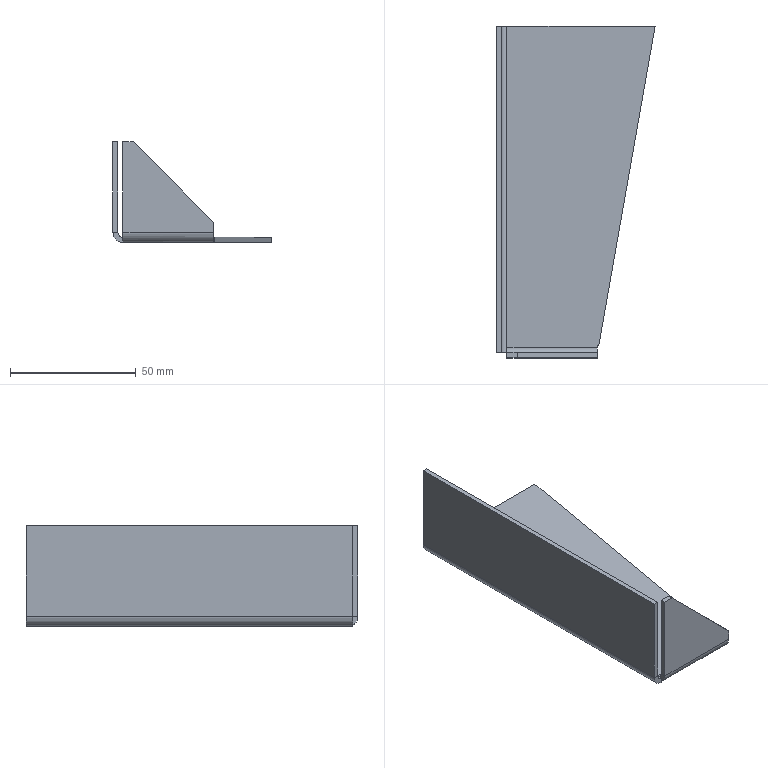Part | SolidWorks | features Chamfer 1, EdgeFlange 1, Extrusion 1, FlatPattern 1, ICE 1, MirrorSolid 1, SheetMetal 1, Shell 1, SolidToSheetMetal 1 | 1 solid | 26 faces | box 62.923 x 132 x 40 mm | volume 24687 mm3 | plane 22 | cylinder 4 | commonest cylinder face diameters 4 x2 8 x2
STEP:
#1=CARTESIAN_POINT('',(-52.191,99.057,0.));
#2=VERTEX_POINT('',#1);
#3=CARTESIAN_POINT('',(-54.191,99.057,0.));
#4=VERTEX_POINT('',#3);
#5=CARTESIAN_POINT('',(-54.191,99.057,0.));
#6=DIRECTION('',(-1.,0.,0.));
#7=VECTOR('',#6,1000.);
#8=LINE('',#5,#7);
#9=EDGE_CURVE('',#2,#4,#8,.T.);
#10=ORIENTED_EDGE('',*,*,#9,.F.);
#11=CARTESIAN_POINT('',(-52.191,99.057,-36.));
#12=VERTEX_POINT('',#11);
#13=CARTESIAN_POINT('',(-52.191,99.057,40.));
#14=DIRECTION('',(0.,0.,-1.));
#15=VECTOR('',#14,1000.);
#16=LINE('',#13,#15);
#17=EDGE_CURVE('',#2,#12,#16,.T.);
#18=ORIENTED_EDGE('',*,*,#17,.T.);
#19=CARTESIAN_POINT('',(-54.191,99.057,-36.));
#20=VERTEX_POINT('',#19);
#21=CARTESIAN_POINT('',(-54.191,99.057,-36.));
#22=DIRECTION('',(-1.,0.,0.));
#23=VECTOR('',#22,1000.);
#24=LINE('',#21,#23);
#25=EDGE_CURVE('',#12,#20,#24,.T.);
#26=ORIENTED_EDGE('',*,*,#25,.T.);
#27=CARTESIAN_POINT('',(-54.191,99.057,40.));
#28=DIRECTION('',(0.,0.,-1.));
#29=VECTOR('',#28,1000.);
#30=LINE('',#27,#29);
#31=EDGE_CURVE('',#4,#20,#30,.T.);
#32=ORIENTED_EDGE('',*,*,#31,.F.);
#33=EDGE_LOOP('',(#10,#18,#26,#32));
#34=FACE_OUTER_BOUND('',#33,.T.);
#35=CARTESIAN_POINT('',(-54.191,99.057,40.));
#36=DIRECTION('',(0.,-1.,0.));
#37=DIRECTION('',(0.,0.,-1.));
#38=AXIS2_PLACEMENT_3D('',#35,#36,#37);
#39=PLANE('',#38);
#40=ADVANCED_FACE('',(#34),#39,.F.);
#41=CARTESIAN_POINT('',(-54.191,-30.943,0.));
#42=VERTEX_POINT('',#41);
#43=CARTESIAN_POINT('',(-52.191,-30.943,0.));
#44=VERTEX_POINT('',#43);
#45=CARTESIAN_POINT('',(-54.191,-30.943,0.));
#46=DIRECTION('',(1.,0.,0.));
#47=VECTOR('',#46,1000.);
#48=LINE('',#45,#47);
#49=EDGE_CURVE('',#42,#44,#48,.T.);
#50=ORIENTED_EDGE('',*,*,#49,.F.);
#51=CARTESIAN_POINT('',(-54.191,-30.943,-36.));
#52=VERTEX_POINT('',#51);
#53=CARTESIAN_POINT('',(-54.191,-30.943,40.));
#54=DIRECTION('',(0.,0.,-1.));
#55=VECTOR('',#54,1000.);
#56=LINE('',#53,#55);
#57=EDGE_CURVE('',#42,#52,#56,.T.);
#58=ORIENTED_EDGE('',*,*,#57,.T.);
#59=CARTESIAN_POINT('',(-52.191,-30.943,-36.));
#60=VERTEX_POINT('',#59);
#61=CARTESIAN_POINT('',(-54.191,-30.943,-36.));
#62=DIRECTION('',(-1.,0.,0.));
#63=VECTOR('',#62,1000.);
#64=LINE('',#61,#63);
#65=EDGE_CURVE('',#60,#52,#64,.T.);
#66=ORIENTED_EDGE('',*,*,#65,.F.);
#67=CARTESIAN_POINT('',(-52.191,-30.943,40.));
#68=DIRECTION('',(0.,0.,-1.));
#69=VECTOR('',#68,1000.);
#70=LINE('',#67,#69);
#71=EDGE_CURVE('',#44,#60,#70,.T.);
#72=ORIENTED_EDGE('',*,*,#71,.F.);
#73=EDGE_LOOP('',(#50,#58,#66,#72));
#74=FACE_OUTER_BOUND('',#73,.T.);
#75=CARTESIAN_POINT('',(-54.191,-30.943,40.));
#76=DIRECTION('',(0.,-1.,0.));
#77=DIRECTION('',(0.,0.,-1.));
#78=AXIS2_PLACEMENT_3D('',#75,#76,#77);
#79=PLANE('',#78);
#80=ADVANCED_FACE('',(#74),#79,.T.);
#81=ORIENTED_EDGE('',*,*,#57,.F.);
#82=CARTESIAN_POINT('',(-54.191,126.407,0.));
#83=DIRECTION('',(0.,1.,0.));
#84=VECTOR('',#83,1000.);
#85=LINE('',#82,#84);
#86=EDGE_CURVE('',#42,#4,#85,.T.);
#87=ORIENTED_EDGE('',*,*,#86,.T.);
#88=ORIENTED_EDGE('',*,*,#31,.T.);
#89=CARTESIAN_POINT('',(-54.191,99.057,-36.));
#90=DIRECTION('',(0.,1.,0.));
#91=VECTOR('',#90,1000.);
#92=LINE('',#89,#91);
#93=EDGE_CURVE('',#52,#20,#92,.T.);
#94=ORIENTED_EDGE('',*,*,#93,.F.);
#95=EDGE_LOOP('',(#81,#87,#88,#94));
#96=FACE_OUTER_BOUND('',#95,.T.);
#97=CARTESIAN_POINT('',(-54.191,-30.943,40.));
#98=DIRECTION('',(1.,0.,0.));
#99=DIRECTION('',(0.,0.,-1.));
#100=AXIS2_PLACEMENT_3D('',#97,#98,#99);
#101=PLANE('',#100);
#102=ADVANCED_FACE('',(#96),#101,.F.);
#103=CARTESIAN_POINT('',(-52.191,-30.943,0.));
#104=DIRECTION('',(0.,1.,0.));
#105=VECTOR('',#104,1000.);
#106=LINE('',#103,#105);
#107=EDGE_CURVE('',#44,#2,#106,.T.);
#108=ORIENTED_EDGE('',*,*,#107,.F.);
#109=ORIENTED_EDGE('',*,*,#71,.T.);
#110=CARTESIAN_POINT('',(-52.191,-30.943,-36.));
#111=DIRECTION('',(0.,1.,0.));
#112=VECTOR('',#111,1000.);
#113=LINE('',#110,#112);
#114=EDGE_CURVE('',#60,#12,#113,.T.);
#115=ORIENTED_EDGE('',*,*,#114,.T.);
#116=ORIENTED_EDGE('',*,*,#17,.F.);
#117=EDGE_LOOP('',(#108,#109,#115,#116));
#118=FACE_OUTER_BOUND('',#117,.T.);
#119=CARTESIAN_POINT('',(-52.191,-30.943,40.));
#120=DIRECTION('',(1.,0.,0.));
#121=DIRECTION('',(0.,0.,-1.));
#122=AXIS2_PLACEMENT_3D('',#119,#120,#121);
#123=PLANE('',#122);
#124=ADVANCED_FACE('',(#118),#123,.T.);
#125=CARTESIAN_POINT('',(-50.191,-32.943,0.));
#126=VERTEX_POINT('',#125);
#127=CARTESIAN_POINT('',(-50.191,-32.943,-36.));
#128=VERTEX_POINT('',#127);
#129=CARTESIAN_POINT('',(-50.191,-32.943,0.));
#130=DIRECTION('',(0.,0.,-1.));
#131=VECTOR('',#130,1000.);
#132=LINE('',#129,#131);
#133=EDGE_CURVE('',#126,#128,#132,.T.);
#134=ORIENTED_EDGE('',*,*,#133,.F.);
#135=CARTESIAN_POINT('',(-50.191,-30.943,0.));
#136=VERTEX_POINT('',#135);
#137=CARTESIAN_POINT('',(-50.191,-32.943,0.));
#138=DIRECTION('',(0.,1.,0.));
#139=VECTOR('',#138,1000.);
#140=LINE('',#137,#139);
#141=EDGE_CURVE('',#126,#136,#140,.T.);
#142=ORIENTED_EDGE('',*,*,#141,.T.);
#143=CARTESIAN_POINT('',(-50.191,-30.943,-36.));
#144=VERTEX_POINT('',#143);
#145=CARTESIAN_POINT('',(-50.191,-30.943,0.));
#146=DIRECTION('',(0.,0.,-1.));
#147=VECTOR('',#146,1000.);
#148=LINE('',#145,#147);
#149=EDGE_CURVE('',#136,#144,#148,.T.);
#150=ORIENTED_EDGE('',*,*,#149,.T.);
#151=CARTESIAN_POINT('',(-50.191,-30.943,-36.));
#152=DIRECTION('',(0.,-1.,0.));
#153=VECTOR('',#152,1000.);
#154=LINE('',#151,#153);
#155=EDGE_CURVE('',#144,#128,#154,.T.);
#156=ORIENTED_EDGE('',*,*,#155,.T.);
#157=EDGE_LOOP('',(#134,#142,#150,#156));
#158=FACE_OUTER_BOUND('',#157,.T.);
#159=CARTESIAN_POINT('',(-50.191,-32.943,0.));
#160=DIRECTION('',(1.,0.,0.));
#161=DIRECTION('',(0.,1.,0.));
#162=AXIS2_PLACEMENT_3D('',#159,#160,#161);
#163=PLANE('',#162);
#164=ADVANCED_FACE('',(#158),#163,.F.);
#165=CARTESIAN_POINT('',(-14.191,-30.943,-36.));
#166=VERTEX_POINT('',#165);
#167=CARTESIAN_POINT('',(-14.191,-30.943,-32.));
#168=VERTEX_POINT('',#167);
#169=CARTESIAN_POINT('',(-14.191,-30.943,38.));
#170=DIRECTION('',(0.,0.,1.));
#171=VECTOR('',#170,1000.);
#172=LINE('',#169,#171);
#173=EDGE_CURVE('',#166,#168,#172,.T.);
#174=ORIENTED_EDGE('',*,*,#173,.T.);
#175=CARTESIAN_POINT('',(-14.191,-32.943,-32.));
#176=VERTEX_POINT('',#175);
#177=CARTESIAN_POINT('',(-14.191,-32.943,-32.));
#178=DIRECTION('',(0.,-1.,0.));
#179=VECTOR('',#178,1000.);
#180=LINE('',#177,#179);
#181=EDGE_CURVE('',#168,#176,#180,.T.);
#182=ORIENTED_EDGE('',*,*,#181,.T.);
#183=CARTESIAN_POINT('',(-14.191,-32.943,-36.));
#184=VERTEX_POINT('',#183);
#185=CARTESIAN_POINT('',(-14.191,-32.943,38.));
#186=DIRECTION('',(0.,0.,1.));
#187=VECTOR('',#186,1000.);
#188=LINE('',#185,#187);
#189=EDGE_CURVE('',#184,#176,#188,.T.);
#190=ORIENTED_EDGE('',*,*,#189,.F.);
#191=CARTESIAN_POINT('',(-14.191,-30.943,-36.));
#192=DIRECTION('',(0.,-1.,0.));
#193=VECTOR('',#192,1000.);
#194=LINE('',#191,#193);
#195=EDGE_CURVE('',#166,#184,#194,.T.);
#196=ORIENTED_EDGE('',*,*,#195,.F.);
#197=EDGE_LOOP('',(#174,#182,#190,#196));
#198=FACE_OUTER_BOUND('',#197,.T.);
#199=CARTESIAN_POINT('',(-14.191,-32.943,38.));
#200=DIRECTION('',(-1.,0.,0.));
#201=DIRECTION('',(0.,-1.,0.));
#202=AXIS2_PLACEMENT_3D('',#199,#200,#201);
#203=PLANE('',#202);
#204=ADVANCED_FACE('',(#198),#203,.F.);
#205=ORIENTED_EDGE('',*,*,#189,.T.);
#206=CARTESIAN_POINT('',(-46.191,-32.943,0.));
#207=VERTEX_POINT('',#206);
#208=CARTESIAN_POINT('',(-14.191,-32.943,-32.));
#209=DIRECTION('',(-0.7071,0.,0.7071));
#210=VECTOR('',#209,1000.);
#211=LINE('',#208,#210);
#212=EDGE_CURVE('',#176,#207,#211,.T.);
#213=ORIENTED_EDGE('',*,*,#212,.T.);
#214=CARTESIAN_POINT('',(0.,-32.943,0.));
#215=DIRECTION('',(-1.,0.,0.));
#216=VECTOR('',#215,1000.);
#217=LINE('',#214,#216);
#218=EDGE_CURVE('',#207,#126,#217,.T.);
#219=ORIENTED_EDGE('',*,*,#218,.T.);
#220=ORIENTED_EDGE('',*,*,#133,.T.);
#221=CARTESIAN_POINT('',(0.,-32.943,-36.));
#222=DIRECTION('',(1.,0.,0.));
#223=VECTOR('',#222,1000.);
#224=LINE('',#221,#223);
#225=EDGE_CURVE('',#128,#184,#224,.T.);
#226=ORIENTED_EDGE('',*,*,#225,.T.);
#227=EDGE_LOOP('',(#205,#213,#219,#220,#226));
#228=FACE_OUTER_BOUND('',#227,.T.);
#229=CARTESIAN_POINT('',(0.,-32.943,0.));
#230=DIRECTION('',(0.,1.,0.));
#231=DIRECTION('',(0.,0.,1.));
#232=AXIS2_PLACEMENT_3D('',#229,#230,#231);
#233=PLANE('',#232);
#234=ADVANCED_FACE('',(#228),#233,.F.);
#235=CARTESIAN_POINT('',(-46.191,-30.943,0.));
#236=VERTEX_POINT('',#235);
#237=CARTESIAN_POINT('',(0.,-30.943,0.));
#238=DIRECTION('',(-1.,0.,0.));
#239=VECTOR('',#238,1000.);
#240=LINE('',#237,#239);
#241=EDGE_CURVE('',#236,#136,#240,.T.);
#242=ORIENTED_EDGE('',*,*,#241,.F.);
#243=CARTESIAN_POINT('',(-23.095,-30.943,-23.095));
#244=DIRECTION('',(0.7071,0.,-0.7071));
#245=VECTOR('',#244,1000.);
#246=LINE('',#243,#245);
#247=EDGE_CURVE('',#236,#168,#246,.T.);
#248=ORIENTED_EDGE('',*,*,#247,.T.);
#249=ORIENTED_EDGE('',*,*,#173,.F.);
#250=CARTESIAN_POINT('',(-14.191,-30.943,-36.));
#251=DIRECTION('',(-1.,0.,0.));
#252=VECTOR('',#251,1000.);
#253=LINE('',#250,#252);
#254=EDGE_CURVE('',#166,#144,#253,.T.);
#255=ORIENTED_EDGE('',*,*,#254,.T.);
#256=ORIENTED_EDGE('',*,*,#149,.F.);
#257=EDGE_LOOP('',(#242,#248,#249,#255,#256));
#258=FACE_OUTER_BOUND('',#257,.T.);
#259=CARTESIAN_POINT('',(0.,-30.943,0.));
#260=DIRECTION('',(0.,1.,0.));
#261=DIRECTION('',(0.,0.,1.));
#262=AXIS2_PLACEMENT_3D('',#259,#260,#261);
#263=PLANE('',#262);
#264=ADVANCED_FACE('',(#258),#263,.T.);
#265=CARTESIAN_POINT('',(-50.191,-30.943,-39.464));
#266=VERTEX_POINT('',#265);
#267=CARTESIAN_POINT('',(-50.191,-30.943,-40.));
#268=VERTEX_POINT('',#267);
#269=CARTESIAN_POINT('',(-50.191,-30.943,-40.));
#270=DIRECTION('',(0.,0.,-1.));
#271=VECTOR('',#270,1000.);
#272=LINE('',#269,#271);
#273=EDGE_CURVE('',#266,#268,#272,.T.);
#274=ORIENTED_EDGE('',*,*,#273,.T.);
#275=CARTESIAN_POINT('',(-50.191,-28.943,-40.));
#276=VERTEX_POINT('',#275);
#277=CARTESIAN_POINT('',(-50.191,0.,-40.));
#278=DIRECTION('',(0.,1.,0.));
#279=VECTOR('',#278,1000.);
#280=LINE('',#277,#279);
#281=EDGE_CURVE('',#268,#276,#280,.T.);
#282=ORIENTED_EDGE('',*,*,#281,.T.);
#283=CARTESIAN_POINT('',(-50.191,-28.943,-36.));
#284=DIRECTION('',(1.,0.,0.));
#285=DIRECTION('',(0.,0.,-1.));
#286=AXIS2_PLACEMENT_3D('',#283,#284,#285);
#287=CIRCLE('',#286,4.);
#288=EDGE_CURVE('',#266,#276,#287,.T.);
#289=ORIENTED_EDGE('',*,*,#288,.F.);
#290=EDGE_LOOP('',(#274,#282,#289));
#291=FACE_OUTER_BOUND('',#290,.T.);
#292=CARTESIAN_POINT('',(-50.191,-30.943,-38.));
#293=DIRECTION('',(1.,0.,0.));
#294=DIRECTION('',(0.,0.,1.));
#295=AXIS2_PLACEMENT_3D('',#292,#293,#294);
#296=PLANE('',#295);
#297=ADVANCED_FACE('',(#291),#296,.T.);
#298=CARTESIAN_POINT('',(-13.662,-27.943,-40.));
#299=VERTEX_POINT('',#298);
#300=CARTESIAN_POINT('',(8.732,99.057,-40.));
#301=VERTEX_POINT('',#300);
#302=CARTESIAN_POINT('',(-14.191,-30.943,-40.));
#303=DIRECTION('',(0.1736,0.9848,0.));
#304=VECTOR('',#303,1000.);
#305=LINE('',#302,#304);
#306=EDGE_CURVE('',#299,#301,#305,.T.);
#307=ORIENTED_EDGE('',*,*,#306,.T.);
#308=CARTESIAN_POINT('',(8.732,99.057,-38.));
#309=VERTEX_POINT('',#308);
#310=CARTESIAN_POINT('',(8.732,99.057,-40.));
#311=DIRECTION('',(0.,0.,-1.));
#312=VECTOR('',#311,1000.);
#313=LINE('',#310,#312);
#314=EDGE_CURVE('',#309,#301,#313,.T.);
#315=ORIENTED_EDGE('',*,*,#314,.F.);
#316=CARTESIAN_POINT('',(-13.662,-27.943,-38.));
#317=VERTEX_POINT('',#316);
#318=CARTESIAN_POINT('',(-14.191,-30.943,-38.));
#319=DIRECTION('',(0.1736,0.9848,0.));
#320=VECTOR('',#319,1000.);
#321=LINE('',#318,#320);
#322=EDGE_CURVE('',#317,#309,#321,.T.);
#323=ORIENTED_EDGE('',*,*,#322,.F.);
#324=CARTESIAN_POINT('',(-13.662,-27.943,-40.));
#325=DIRECTION('',(0.,0.,1.));
#326=VECTOR('',#325,1000.);
#327=LINE('',#324,#326);
#328=EDGE_CURVE('',#299,#317,#327,.T.);
#329=ORIENTED_EDGE('',*,*,#328,.F.);
#330=EDGE_LOOP('',(#307,#315,#323,#329));
#331=FACE_OUTER_BOUND('',#330,.T.);
#332=CARTESIAN_POINT('',(-14.191,-30.943,-40.));
#333=DIRECTION('',(0.9848,-0.1736,0.));
#334=DIRECTION('',(0.1736,0.9848,0.));
#335=AXIS2_PLACEMENT_3D('',#332,#333,#334);
#336=PLANE('',#335);
#337=ADVANCED_FACE('',(#331),#336,.T.);
#338=CARTESIAN_POINT('',(-50.191,99.057,-40.));
#339=VERTEX_POINT('',#338);
#340=CARTESIAN_POINT('',(-50.191,-30.943,-40.));
#341=DIRECTION('',(0.,-1.,0.));
#342=VECTOR('',#341,1000.);
#343=LINE('',#340,#342);
#344=EDGE_CURVE('',#339,#276,#343,.T.);
#345=ORIENTED_EDGE('',*,*,#344,.F.);
#346=CARTESIAN_POINT('',(8.732,99.057,-40.));
#347=DIRECTION('',(-1.,0.,0.));
#348=VECTOR('',#347,1000.);
#349=LINE('',#346,#348);
#350=EDGE_CURVE('',#301,#339,#349,.T.);
#351=ORIENTED_EDGE('',*,*,#350,.F.);
#352=ORIENTED_EDGE('',*,*,#306,.F.);
#353=CARTESIAN_POINT('',(-14.191,-27.943,-40.));
#354=VERTEX_POINT('',#353);
#355=CARTESIAN_POINT('',(0.,-27.943,-40.));
#356=DIRECTION('',(1.,0.,0.));
#357=VECTOR('',#356,1000.);
#358=LINE('',#355,#357);
#359=EDGE_CURVE('',#354,#299,#358,.T.);
#360=ORIENTED_EDGE('',*,*,#359,.F.);
#361=CARTESIAN_POINT('',(-14.191,-28.943,-40.));
#362=VERTEX_POINT('',#361);
#363=CARTESIAN_POINT('',(-14.191,0.,-40.));
#364=DIRECTION('',(0.,1.,0.));
#365=VECTOR('',#364,1000.);
#366=LINE('',#363,#365);
#367=EDGE_CURVE('',#362,#354,#366,.T.);
#368=ORIENTED_EDGE('',*,*,#367,.F.);
#369=CARTESIAN_POINT('',(-50.191,-28.943,-40.));
#370=DIRECTION('',(1.,0.,0.));
#371=VECTOR('',#370,1000.);
#372=LINE('',#369,#371);
#373=EDGE_CURVE('',#276,#362,#372,.T.);
#374=ORIENTED_EDGE('',*,*,#373,.F.);
#375=EDGE_LOOP('',(#345,#351,#352,#360,#368,#374));
#376=FACE_OUTER_BOUND('',#375,.T.);
#377=CARTESIAN_POINT('',(0.,0.,-40.));
#378=DIRECTION('',(0.,0.,-1.));
#379=DIRECTION('',(1.,0.,0.));
#380=AXIS2_PLACEMENT_3D('',#377,#378,#379);
#381=PLANE('',#380);
#382=ADVANCED_FACE('',(#376),#381,.T.);
#383=CARTESIAN_POINT('',(-50.191,-28.943,-38.));
#384=VERTEX_POINT('',#383);
#385=CARTESIAN_POINT('',(-14.191,-28.943,-38.));
#386=VERTEX_POINT('',#385);
#387=CARTESIAN_POINT('',(-50.191,-28.943,-38.));
#388=DIRECTION('',(1.,0.,0.));
#389=VECTOR('',#388,1000.);
#390=LINE('',#387,#389);
#391=EDGE_CURVE('',#384,#386,#390,.T.);
#392=ORIENTED_EDGE('',*,*,#391,.T.);
#393=CARTESIAN_POINT('',(-14.191,-27.943,-38.));
#394=VERTEX_POINT('',#393);
#395=CARTESIAN_POINT('',(-14.191,-28.943,-38.));
#396=DIRECTION('',(0.,1.,0.));
#397=VECTOR('',#396,1000.);
#398=LINE('',#395,#397);
#399=EDGE_CURVE('',#386,#394,#398,.T.);
#400=ORIENTED_EDGE('',*,*,#399,.T.);
#401=CARTESIAN_POINT('',(-14.191,-27.943,-38.));
#402=DIRECTION('',(1.,0.,0.));
#403=VECTOR('',#402,1000.);
#404=LINE('',#401,#403);
#405=EDGE_CURVE('',#394,#317,#404,.T.);
#406=ORIENTED_EDGE('',*,*,#405,.T.);
#407=ORIENTED_EDGE('',*,*,#322,.T.);
#408=CARTESIAN_POINT('',(-50.191,99.057,-38.));
#409=VERTEX_POINT('',#408);
#410=CARTESIAN_POINT('',(0.,99.057,-38.));
#411=DIRECTION('',(-1.,0.,0.));
#412=VECTOR('',#411,1000.);
#413=LINE('',#410,#412);
#414=EDGE_CURVE('',#309,#409,#413,.T.);
#415=ORIENTED_EDGE('',*,*,#414,.T.);
#416=CARTESIAN_POINT('',(-50.191,0.,-38.));
#417=DIRECTION('',(0.,-1.,0.));
#418=VECTOR('',#417,1000.);
#419=LINE('',#416,#418);
#420=EDGE_CURVE('',#409,#384,#419,.T.);
#421=ORIENTED_EDGE('',*,*,#420,.T.);
#422=EDGE_LOOP('',(#392,#400,#406,#407,#415,#421));
#423=FACE_OUTER_BOUND('',#422,.T.);
#424=CARTESIAN_POINT('',(0.,0.,-38.));
#425=DIRECTION('',(0.,0.,-1.));
#426=DIRECTION('',(1.,0.,0.));
#427=AXIS2_PLACEMENT_3D('',#424,#425,#426);
#428=PLANE('',#427);
#429=ADVANCED_FACE('',(#423),#428,.F.);
#430=ORIENTED_EDGE('',*,*,#314,.T.);
#431=ORIENTED_EDGE('',*,*,#350,.T.);
#432=CARTESIAN_POINT('',(-50.191,99.057,-40.));
#433=DIRECTION('',(0.,0.,-1.));
#434=VECTOR('',#433,1000.);
#435=LINE('',#432,#434);
#436=EDGE_CURVE('',#409,#339,#435,.T.);
#437=ORIENTED_EDGE('',*,*,#436,.F.);
#438=ORIENTED_EDGE('',*,*,#414,.F.);
#439=EDGE_LOOP('',(#430,#431,#437,#438));
#440=FACE_OUTER_BOUND('',#439,.T.);
#441=CARTESIAN_POINT('',(8.732,99.057,-40.));
#442=DIRECTION('',(0.,1.,0.));
#443=DIRECTION('',(-1.,0.,0.));
#444=AXIS2_PLACEMENT_3D('',#441,#442,#443);
#445=PLANE('',#444);
#446=ADVANCED_FACE('',(#440),#445,.T.);
#447=ORIENTED_EDGE('',*,*,#436,.T.);
#448=CARTESIAN_POINT('',(-50.191,99.057,-36.));
#449=DIRECTION('',(0.,1.,0.));
#450=DIRECTION('',(0.,0.,-1.));
#451=AXIS2_PLACEMENT_3D('',#448,#449,#450);
#452=CIRCLE('',#451,4.);
#453=EDGE_CURVE('',#339,#20,#452,.T.);
#454=ORIENTED_EDGE('',*,*,#453,.T.);
#455=ORIENTED_EDGE('',*,*,#25,.F.);
#456=CARTESIAN_POINT('',(-50.191,99.057,-36.));
#457=DIRECTION('',(0.,1.,0.));
#458=DIRECTION('',(0.,0.,-1.));
#459=AXIS2_PLACEMENT_3D('',#456,#457,#458);
#460=CIRCLE('',#459,2.);
#461=EDGE_CURVE('',#409,#12,#460,.T.);
#462=ORIENTED_EDGE('',*,*,#461,.F.);
#463=EDGE_LOOP('',(#447,#454,#455,#462));
#464=FACE_OUTER_BOUND('',#463,.T.);
#465=CARTESIAN_POINT('',(-50.191,99.057,-36.));
#466=DIRECTION('',(0.,-1.,0.));
#467=DIRECTION('',(0.,0.,1.));
#468=AXIS2_PLACEMENT_3D('',#465,#466,#467);
#469=PLANE('',#468);
#470=ADVANCED_FACE('',(#464),#469,.F.);
#471=CARTESIAN_POINT('',(-50.191,-30.943,-38.));
#472=VERTEX_POINT('',#471);
#473=CARTESIAN_POINT('',(-50.191,-30.943,-36.));
#474=DIRECTION('',(0.,-1.,0.));
#475=DIRECTION('',(0.,0.,-1.));
#476=AXIS2_PLACEMENT_3D('',#473,#474,#475);
#477=CIRCLE('',#476,2.);
#478=EDGE_CURVE('',#60,#472,#477,.T.);
#479=ORIENTED_EDGE('',*,*,#478,.F.);
#480=ORIENTED_EDGE('',*,*,#65,.T.);
#481=CARTESIAN_POINT('',(-50.191,-30.943,-36.));
#482=DIRECTION('',(0.,-1.,0.));
#483=DIRECTION('',(0.,0.,-1.));
#484=AXIS2_PLACEMENT_3D('',#481,#482,#483);
#485=CIRCLE('',#484,4.);
#486=EDGE_CURVE('',#52,#268,#485,.T.);
#487=ORIENTED_EDGE('',*,*,#486,.T.);
#488=ORIENTED_EDGE('',*,*,#273,.F.);
#489=CARTESIAN_POINT('',(-50.191,-30.943,-40.));
#490=DIRECTION('',(0.,0.,-1.));
#491=VECTOR('',#490,1000.);
#492=LINE('',#489,#491);
#493=EDGE_CURVE('',#472,#266,#492,.T.);
#494=ORIENTED_EDGE('',*,*,#493,.F.);
#495=EDGE_LOOP('',(#479,#480,#487,#488,#494));
#496=FACE_OUTER_BOUND('',#495,.T.);
#497=CARTESIAN_POINT('',(-50.191,-30.943,-36.));
#498=DIRECTION('',(0.,-1.,0.));
#499=DIRECTION('',(0.,0.,1.));
#500=AXIS2_PLACEMENT_3D('',#497,#498,#499);
#501=PLANE('',#500);
#502=ADVANCED_FACE('',(#496),#501,.T.);
#503=ORIENTED_EDGE('',*,*,#453,.F.);
#504=ORIENTED_EDGE('',*,*,#344,.T.);
#505=ORIENTED_EDGE('',*,*,#281,.F.);
#506=ORIENTED_EDGE('',*,*,#486,.F.);
#507=ORIENTED_EDGE('',*,*,#93,.T.);
#508=EDGE_LOOP('',(#503,#504,#505,#506,#507));
#509=FACE_OUTER_BOUND('',#508,.T.);
#510=CARTESIAN_POINT('',(-50.191,0.,-36.));
#511=DIRECTION('',(0.,1.,0.));
#512=DIRECTION('',(0.,0.,-1.));
#513=AXIS2_PLACEMENT_3D('',#510,#511,#512);
#514=CYLINDRICAL_SURFACE('',#513,4.);
#515=ADVANCED_FACE('',(#509),#514,.T.);
#516=ORIENTED_EDGE('',*,*,#461,.T.);
#517=ORIENTED_EDGE('',*,*,#114,.F.);
#518=ORIENTED_EDGE('',*,*,#478,.T.);
#519=CARTESIAN_POINT('',(-50.191,-30.943,-38.));
#520=DIRECTION('',(0.,1.,0.));
#521=VECTOR('',#520,1000.);
#522=LINE('',#519,#521);
#523=EDGE_CURVE('',#472,#384,#522,.T.);
#524=ORIENTED_EDGE('',*,*,#523,.T.);
#525=ORIENTED_EDGE('',*,*,#420,.F.);
#526=EDGE_LOOP('',(#516,#517,#518,#524,#525));
#527=FACE_OUTER_BOUND('',#526,.T.);
#528=CARTESIAN_POINT('',(-50.191,0.,-36.));
#529=DIRECTION('',(0.,1.,0.));
#530=DIRECTION('',(0.,0.,-1.));
#531=AXIS2_PLACEMENT_3D('',#528,#529,#530);
#532=CYLINDRICAL_SURFACE('',#531,2.);
#533=ADVANCED_FACE('',(#527),#532,.F.);
#534=ORIENTED_EDGE('',*,*,#367,.T.);
#535=CARTESIAN_POINT('',(-14.191,-27.943,-38.));
#536=DIRECTION('',(0.,0.,-1.));
#537=VECTOR('',#536,1000.);
#538=LINE('',#535,#537);
#539=EDGE_CURVE('',#394,#354,#538,.T.);
#540=ORIENTED_EDGE('',*,*,#539,.F.);
#541=ORIENTED_EDGE('',*,*,#399,.F.);
#542=CARTESIAN_POINT('',(-14.191,-28.943,-38.));
#543=DIRECTION('',(0.,0.,-1.));
#544=VECTOR('',#543,1000.);
#545=LINE('',#542,#544);
#546=EDGE_CURVE('',#386,#362,#545,.T.);
#547=ORIENTED_EDGE('',*,*,#546,.T.);
#548=EDGE_LOOP('',(#534,#540,#541,#547));
#549=FACE_OUTER_BOUND('',#548,.T.);
#550=CARTESIAN_POINT('',(-14.191,-28.943,-38.));
#551=DIRECTION('',(1.,0.,0.));
#552=DIRECTION('',(0.,0.,1.));
#553=AXIS2_PLACEMENT_3D('',#550,#551,#552);
#554=PLANE('',#553);
#555=ADVANCED_FACE('',(#549),#554,.T.);
#556=ORIENTED_EDGE('',*,*,#328,.T.);
#557=ORIENTED_EDGE('',*,*,#405,.F.);
#558=ORIENTED_EDGE('',*,*,#539,.T.);
#559=ORIENTED_EDGE('',*,*,#359,.T.);
#560=EDGE_LOOP('',(#556,#557,#558,#559));
#561=FACE_OUTER_BOUND('',#560,.T.);
#562=CARTESIAN_POINT('',(-14.191,-27.943,-38.));
#563=DIRECTION('',(0.,-1.,0.));
#564=DIRECTION('',(0.,0.,1.));
#565=AXIS2_PLACEMENT_3D('',#562,#563,#564);
#566=PLANE('',#565);
#567=ADVANCED_FACE('',(#561),#566,.T.);
#568=ORIENTED_EDGE('',*,*,#493,.T.);
#569=CARTESIAN_POINT('',(-50.191,-28.943,-36.));
#570=DIRECTION('',(1.,0.,0.));
#571=DIRECTION('',(0.,0.,-1.));
#572=AXIS2_PLACEMENT_3D('',#569,#570,#571);
#573=CIRCLE('',#572,4.);
#574=EDGE_CURVE('',#128,#266,#573,.T.);
#575=ORIENTED_EDGE('',*,*,#574,.F.);
#576=ORIENTED_EDGE('',*,*,#155,.F.);
#577=CARTESIAN_POINT('',(-50.191,-28.943,-36.));
#578=DIRECTION('',(1.,0.,0.));
#579=DIRECTION('',(0.,0.,-1.));
#580=AXIS2_PLACEMENT_3D('',#577,#578,#579);
#581=CIRCLE('',#580,2.);
#582=EDGE_CURVE('',#144,#384,#581,.T.);
#583=ORIENTED_EDGE('',*,*,#582,.T.);
#584=ORIENTED_EDGE('',*,*,#523,.F.);
#585=EDGE_LOOP('',(#568,#575,#576,#583,#584));
#586=FACE_OUTER_BOUND('',#585,.T.);
#587=CARTESIAN_POINT('',(-50.191,-28.943,-36.));
#588=DIRECTION('',(1.,0.,0.));
#589=DIRECTION('',(0.,0.,1.));
#590=AXIS2_PLACEMENT_3D('',#587,#588,#589);
#591=PLANE('',#590);
#592=ADVANCED_FACE('',(#586),#591,.F.);
#593=ORIENTED_EDGE('',*,*,#195,.T.);
#594=CARTESIAN_POINT('',(-14.191,-28.943,-36.));
#595=DIRECTION('',(-1.,0.,0.));
#596=DIRECTION('',(0.,0.,-1.));
#597=AXIS2_PLACEMENT_3D('',#594,#595,#596);
#598=CIRCLE('',#597,4.);
#599=EDGE_CURVE('',#362,#184,#598,.T.);
#600=ORIENTED_EDGE('',*,*,#599,.F.);
#601=ORIENTED_EDGE('',*,*,#546,.F.);
#602=CARTESIAN_POINT('',(-14.191,-28.943,-36.));
#603=DIRECTION('',(-1.,0.,0.));
#604=DIRECTION('',(0.,0.,-1.));
#605=AXIS2_PLACEMENT_3D('',#602,#603,#604);
#606=CIRCLE('',#605,2.);
#607=EDGE_CURVE('',#386,#166,#606,.T.);
#608=ORIENTED_EDGE('',*,*,#607,.T.);
#609=EDGE_LOOP('',(#593,#600,#601,#608));
#610=FACE_OUTER_BOUND('',#609,.T.);
#611=CARTESIAN_POINT('',(-14.191,-28.943,-36.));
#612=DIRECTION('',(1.,0.,0.));
#613=DIRECTION('',(0.,0.,1.));
#614=AXIS2_PLACEMENT_3D('',#611,#612,#613);
#615=PLANE('',#614);
#616=ADVANCED_FACE('',(#610),#615,.T.);
#617=ORIENTED_EDGE('',*,*,#373,.T.);
#618=ORIENTED_EDGE('',*,*,#599,.T.);
#619=ORIENTED_EDGE('',*,*,#225,.F.);
#620=ORIENTED_EDGE('',*,*,#574,.T.);
#621=ORIENTED_EDGE('',*,*,#288,.T.);
#622=EDGE_LOOP('',(#617,#618,#619,#620,#621));
#623=FACE_OUTER_BOUND('',#622,.T.);
#624=CARTESIAN_POINT('',(-50.191,-28.943,-36.));
#625=DIRECTION('',(-1.,0.,0.));
#626=DIRECTION('',(0.,-1.,0.));
#627=AXIS2_PLACEMENT_3D('',#624,#625,#626);
#628=CYLINDRICAL_SURFACE('',#627,4.);
#629=ADVANCED_FACE('',(#623),#628,.T.);
#630=ORIENTED_EDGE('',*,*,#391,.F.);
#631=ORIENTED_EDGE('',*,*,#582,.F.);
#632=ORIENTED_EDGE('',*,*,#254,.F.);
#633=ORIENTED_EDGE('',*,*,#607,.F.);
#634=EDGE_LOOP('',(#630,#631,#632,#633));
#635=FACE_OUTER_BOUND('',#634,.T.);
#636=CARTESIAN_POINT('',(-50.191,-28.943,-36.));
#637=DIRECTION('',(-1.,0.,0.));
#638=DIRECTION('',(0.,-1.,0.));
#639=AXIS2_PLACEMENT_3D('',#636,#637,#638);
#640=CYLINDRICAL_SURFACE('',#639,2.);
#641=ADVANCED_FACE('',(#635),#640,.F.);
#642=ORIENTED_EDGE('',*,*,#218,.F.);
#643=CARTESIAN_POINT('',(-46.191,126.407,0.));
#644=DIRECTION('',(0.,1.,0.));
#645=VECTOR('',#644,1000.);
#646=LINE('',#643,#645);
#647=EDGE_CURVE('',#207,#236,#646,.T.);
#648=ORIENTED_EDGE('',*,*,#647,.T.);
#649=ORIENTED_EDGE('',*,*,#241,.T.);
#650=ORIENTED_EDGE('',*,*,#141,.F.);
#651=EDGE_LOOP('',(#642,#648,#649,#650));
#652=FACE_OUTER_BOUND('',#651,.T.);
#653=CARTESIAN_POINT('',(-54.191,126.407,0.));
#654=DIRECTION('',(0.,0.,-1.));
#655=DIRECTION('',(-1.,0.,0.));
#656=AXIS2_PLACEMENT_3D('',#653,#654,#655);
#657=PLANE('',#656);
#658=ADVANCED_FACE('',(#652),#657,.F.);
#659=ORIENTED_EDGE('',*,*,#9,.T.);
#660=ORIENTED_EDGE('',*,*,#86,.F.);
#661=ORIENTED_EDGE('',*,*,#49,.T.);
#662=ORIENTED_EDGE('',*,*,#107,.T.);
#663=EDGE_LOOP('',(#659,#660,#661,#662));
#664=FACE_OUTER_BOUND('',#663,.T.);
#665=CARTESIAN_POINT('',(-54.191,126.407,0.));
#666=DIRECTION('',(0.,0.,-1.));
#667=DIRECTION('',(-1.,0.,0.));
#668=AXIS2_PLACEMENT_3D('',#665,#666,#667);
#669=PLANE('',#668);
#670=ADVANCED_FACE('',(#664),#669,.F.);
#671=ORIENTED_EDGE('',*,*,#247,.F.);
#672=ORIENTED_EDGE('',*,*,#647,.F.);
#673=ORIENTED_EDGE('',*,*,#212,.F.);
#674=ORIENTED_EDGE('',*,*,#181,.F.);
#675=EDGE_LOOP('',(#671,#672,#673,#674));
#676=FACE_OUTER_BOUND('',#675,.T.);
#677=CARTESIAN_POINT('',(-14.191,-32.943,-32.));
#678=DIRECTION('',(-0.7071,0.,-0.7071));
#679=DIRECTION('',(0.,-1.,0.));
#680=AXIS2_PLACEMENT_3D('',#677,#678,#679);
#681=PLANE('',#680);
#682=ADVANCED_FACE('',(#676),#681,.F.);
#683=CLOSED_SHELL('',(#40,#80,#102,#124,#164,#204,#234,#264,#297,#337,#382,#429,#446,#470,#502,#515,#533,#555,#567,#592,#616,#629,#641,#658,#670,#682));
#684=MANIFOLD_SOLID_BREP('',#683);
#685=CARTESIAN_POINT('',(0.,0.,0.));
#686=DIRECTION('',(0.,0.,1.));
#687=DIRECTION('',(1.,0.,0.));
#688=AXIS2_PLACEMENT_3D('',#685,#686,#687);
#689=(LENGTH_UNIT()NAMED_UNIT(*)SI_UNIT(.MILLI.,.METRE.));
#690=UNCERTAINTY_MEASURE_WITH_UNIT(LENGTH_MEASURE(0.00001),#689,'','');
#691=(NAMED_UNIT(*)PLANE_ANGLE_UNIT()SI_UNIT($,.RADIAN.));
#692=(NAMED_UNIT(*)SI_UNIT($,.STERADIAN.)SOLID_ANGLE_UNIT());
#693=(GEOMETRIC_REPRESENTATION_CONTEXT(3)GLOBAL_UNCERTAINTY_ASSIGNED_CONTEXT((#690))GLOBAL_UNIT_ASSIGNED_CONTEXT((#689,#691,#692))REPRESENTATION_CONTEXT('',''));
#694=ADVANCED_BREP_SHAPE_REPRESENTATION('',(#684,#688),#693);